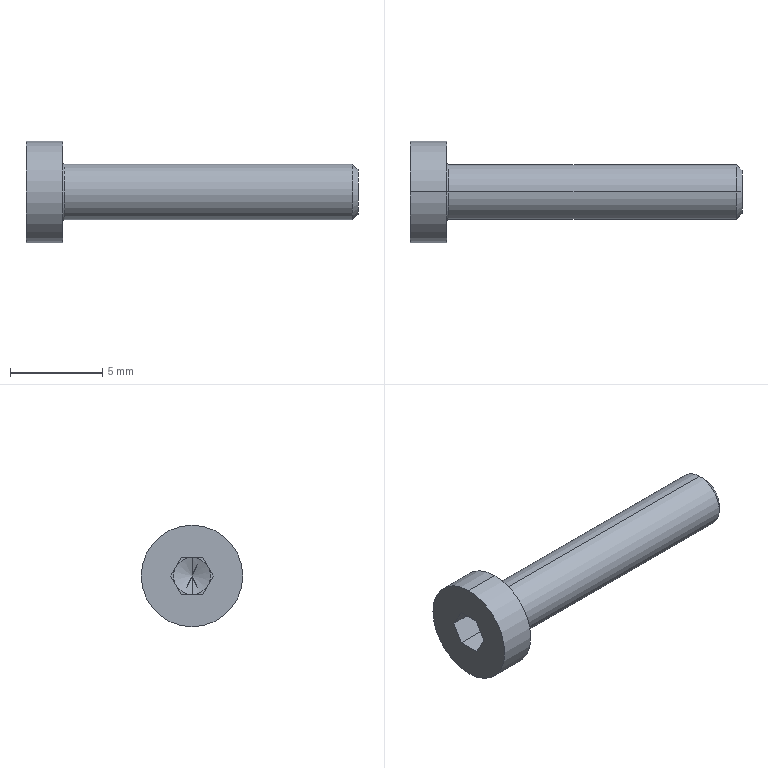Part | SolidWorks | features ICE 1, RevCut 1, Revolution 1 | 1 solid | 25 faces | box 18 x 5.5 x 5.5 mm | volume 154.645 mm3 | plane 15 | cone 4 | cylinder 4 | torus 2 | commonest cylinder face diameters 3 x2 5.5 x2
STEP:
#1=CARTESIAN_POINT('',(-0.136,0.,0.));
#2=VERTEX_POINT('',#1);
#3=CARTESIAN_POINT('',(-0.5,0.,1.));
#4=VERTEX_POINT('',#3);
#5=CARTESIAN_POINT('',(-0.136,0.,0.));
#6=DIRECTION('',(-0.342,0.,0.9397));
#7=VECTOR('',#6,1000.);
#8=LINE('',#5,#7);
#9=EDGE_CURVE('',#2,#4,#8,.T.);
#10=ORIENTED_EDGE('',*,*,#9,.F.);
#11=CARTESIAN_POINT('',(-0.5,0.,-1.));
#12=VERTEX_POINT('',#11);
#13=CARTESIAN_POINT('',(-0.136,0.,0.));
#14=DIRECTION('',(-0.342,0.,-0.9397));
#15=VECTOR('',#14,1000.);
#16=LINE('',#13,#15);
#17=EDGE_CURVE('',#2,#12,#16,.T.);
#18=ORIENTED_EDGE('',*,*,#17,.T.);
#19=CARTESIAN_POINT('',(-0.5,-0.866,-0.5));
#20=VERTEX_POINT('',#19);
#21=CARTESIAN_POINT('',(-0.5,0.,0.));
#22=DIRECTION('',(-1.,0.,0.));
#23=DIRECTION('',(0.,0.,1.));
#24=AXIS2_PLACEMENT_3D('',#21,#22,#23);
#25=CIRCLE('',#24,1.);
#26=EDGE_CURVE('',#12,#20,#25,.T.);
#27=ORIENTED_EDGE('',*,*,#26,.T.);
#28=CARTESIAN_POINT('',(-0.5,-0.866,0.5));
#29=VERTEX_POINT('',#28);
#30=CARTESIAN_POINT('',(-0.5,0.,0.));
#31=DIRECTION('',(-1.,0.,0.));
#32=DIRECTION('',(0.,0.,1.));
#33=AXIS2_PLACEMENT_3D('',#30,#31,#32);
#34=CIRCLE('',#33,1.);
#35=EDGE_CURVE('',#20,#29,#34,.T.);
#36=ORIENTED_EDGE('',*,*,#35,.T.);
#37=CARTESIAN_POINT('',(-0.5,0.,0.));
#38=DIRECTION('',(-1.,0.,0.));
#39=DIRECTION('',(0.,0.,1.));
#40=AXIS2_PLACEMENT_3D('',#37,#38,#39);
#41=CIRCLE('',#40,1.);
#42=EDGE_CURVE('',#29,#4,#41,.T.);
#43=ORIENTED_EDGE('',*,*,#42,.T.);
#44=EDGE_LOOP('',(#10,#18,#27,#36,#43));
#45=FACE_OUTER_BOUND('',#44,.T.);
#46=CARTESIAN_POINT('',(-1000.136,0.,0.));
#47=DIRECTION('',(-1.,0.,0.));
#48=DIRECTION('',(0.,0.,1.));
#49=AXIS2_PLACEMENT_3D('',#46,#47,#48);
#50=CONICAL_SURFACE('',#49,2747.477,1.222);
#51=ADVANCED_FACE('',(#45),#50,.F.);
#52=CARTESIAN_POINT('',(0.,0.,2.75));
#53=VERTEX_POINT('',#52);
#54=CARTESIAN_POINT('',(0.,0.,-2.75));
#55=VERTEX_POINT('',#54);
#56=CARTESIAN_POINT('',(0.,0.,0.));
#57=DIRECTION('',(-1.,0.,0.));
#58=DIRECTION('',(0.,0.,1.));
#59=AXIS2_PLACEMENT_3D('',#56,#57,#58);
#60=CIRCLE('',#59,2.75);
#61=EDGE_CURVE('',#53,#55,#60,.T.);
#62=ORIENTED_EDGE('',*,*,#61,.T.);
#63=CARTESIAN_POINT('',(-2.,0.,-2.75));
#64=VERTEX_POINT('',#63);
#65=CARTESIAN_POINT('',(16.,0.,-2.75));
#66=DIRECTION('',(-1.,0.,0.));
#67=VECTOR('',#66,1000.);
#68=LINE('',#65,#67);
#69=EDGE_CURVE('',#55,#64,#68,.T.);
#70=ORIENTED_EDGE('',*,*,#69,.T.);
#71=CARTESIAN_POINT('',(-2.,0.,2.75));
#72=VERTEX_POINT('',#71);
#73=CARTESIAN_POINT('',(-2.,0.,0.));
#74=DIRECTION('',(-1.,0.,0.));
#75=DIRECTION('',(0.,0.,1.));
#76=AXIS2_PLACEMENT_3D('',#73,#74,#75);
#77=CIRCLE('',#76,2.75);
#78=EDGE_CURVE('',#72,#64,#77,.T.);
#79=ORIENTED_EDGE('',*,*,#78,.F.);
#80=CARTESIAN_POINT('',(16.,0.,2.75));
#81=DIRECTION('',(-1.,0.,0.));
#82=VECTOR('',#81,1000.);
#83=LINE('',#80,#82);
#84=EDGE_CURVE('',#53,#72,#83,.T.);
#85=ORIENTED_EDGE('',*,*,#84,.F.);
#86=EDGE_LOOP('',(#62,#70,#79,#85));
#87=FACE_OUTER_BOUND('',#86,.T.);
#88=CARTESIAN_POINT('',(16.,0.,0.));
#89=DIRECTION('',(-1.,0.,0.));
#90=DIRECTION('',(0.,0.,1.));
#91=AXIS2_PLACEMENT_3D('',#88,#89,#90);
#92=CYLINDRICAL_SURFACE('',#91,2.75);
#93=ADVANCED_FACE('',(#87),#92,.T.);
#94=CARTESIAN_POINT('',(0.,0.,-1.6));
#95=VERTEX_POINT('',#94);
#96=CARTESIAN_POINT('',(0.,0.,1.6));
#97=VERTEX_POINT('',#96);
#98=CARTESIAN_POINT('',(0.,0.,0.));
#99=DIRECTION('',(-1.,0.,0.));
#100=DIRECTION('',(0.,0.,1.));
#101=AXIS2_PLACEMENT_3D('',#98,#99,#100);
#102=CIRCLE('',#101,1.6);
#103=EDGE_CURVE('',#95,#97,#102,.T.);
#104=ORIENTED_EDGE('',*,*,#103,.F.);
#105=CARTESIAN_POINT('',(0.1,0.,-1.5));
#106=VERTEX_POINT('',#105);
#107=CARTESIAN_POINT('',(0.1,0.,-1.6));
#108=DIRECTION('',(0.,1.,0.));
#109=DIRECTION('',(0.,0.,1.));
#110=AXIS2_PLACEMENT_3D('',#107,#108,#109);
#111=CIRCLE('',#110,0.1);
#112=EDGE_CURVE('',#95,#106,#111,.T.);
#113=ORIENTED_EDGE('',*,*,#112,.T.);
#114=CARTESIAN_POINT('',(0.1,0.,1.5));
#115=VERTEX_POINT('',#114);
#116=CARTESIAN_POINT('',(0.1,0.,0.));
#117=DIRECTION('',(-1.,0.,0.));
#118=DIRECTION('',(0.,0.,1.));
#119=AXIS2_PLACEMENT_3D('',#116,#117,#118);
#120=CIRCLE('',#119,1.5);
#121=EDGE_CURVE('',#106,#115,#120,.T.);
#122=ORIENTED_EDGE('',*,*,#121,.T.);
#123=CARTESIAN_POINT('',(0.1,0.,1.6));
#124=DIRECTION('',(0.,-1.,0.));
#125=DIRECTION('',(0.,0.,-1.));
#126=AXIS2_PLACEMENT_3D('',#123,#124,#125);
#127=CIRCLE('',#126,0.1);
#128=EDGE_CURVE('',#97,#115,#127,.T.);
#129=ORIENTED_EDGE('',*,*,#128,.F.);
#130=EDGE_LOOP('',(#104,#113,#122,#129));
#131=FACE_OUTER_BOUND('',#130,.T.);
#132=CARTESIAN_POINT('',(0.1,0.,0.));
#133=DIRECTION('',(-1.,0.,0.));
#134=DIRECTION('',(0.,0.,1.));
#135=AXIS2_PLACEMENT_3D('',#132,#133,#134);
#136=TOROIDAL_SURFACE('',#135,1.6,0.1);
#137=ADVANCED_FACE('',(#131),#136,.F.);
#138=CARTESIAN_POINT('',(15.693,0.,1.5));
#139=VERTEX_POINT('',#138);
#140=CARTESIAN_POINT('',(15.693,0.,-1.5));
#141=VERTEX_POINT('',#140);
#142=CARTESIAN_POINT('',(15.693,0.,0.));
#143=DIRECTION('',(-1.,0.,0.));
#144=DIRECTION('',(0.,0.,1.));
#145=AXIS2_PLACEMENT_3D('',#142,#143,#144);
#146=CIRCLE('',#145,1.5);
#147=EDGE_CURVE('',#139,#141,#146,.T.);
#148=ORIENTED_EDGE('',*,*,#147,.T.);
#149=CARTESIAN_POINT('',(16.,0.,-1.5));
#150=DIRECTION('',(-1.,0.,0.));
#151=VECTOR('',#150,1000.);
#152=LINE('',#149,#151);
#153=EDGE_CURVE('',#141,#106,#152,.T.);
#154=ORIENTED_EDGE('',*,*,#153,.T.);
#155=CARTESIAN_POINT('',(0.1,0.,0.));
#156=DIRECTION('',(-1.,0.,0.));
#157=DIRECTION('',(0.,0.,1.));
#158=AXIS2_PLACEMENT_3D('',#155,#156,#157);
#159=CIRCLE('',#158,1.5);
#160=EDGE_CURVE('',#115,#106,#159,.T.);
#161=ORIENTED_EDGE('',*,*,#160,.F.);
#162=CARTESIAN_POINT('',(16.,0.,1.5));
#163=DIRECTION('',(-1.,0.,0.));
#164=VECTOR('',#163,1000.);
#165=LINE('',#162,#164);
#166=EDGE_CURVE('',#139,#115,#165,.T.);
#167=ORIENTED_EDGE('',*,*,#166,.F.);
#168=EDGE_LOOP('',(#148,#154,#161,#167));
#169=FACE_OUTER_BOUND('',#168,.T.);
#170=CARTESIAN_POINT('',(16.,0.,0.));
#171=DIRECTION('',(-1.,0.,0.));
#172=DIRECTION('',(0.,0.,1.));
#173=AXIS2_PLACEMENT_3D('',#170,#171,#172);
#174=CYLINDRICAL_SURFACE('',#173,1.5);
#175=ADVANCED_FACE('',(#169),#174,.T.);
#176=CARTESIAN_POINT('',(16.,0.,1.194));
#177=VERTEX_POINT('',#176);
#178=CARTESIAN_POINT('',(16.,0.,-1.194));
#179=VERTEX_POINT('',#178);
#180=CARTESIAN_POINT('',(16.,0.,0.));
#181=DIRECTION('',(-1.,0.,0.));
#182=DIRECTION('',(0.,0.,1.));
#183=AXIS2_PLACEMENT_3D('',#180,#181,#182);
#184=CIRCLE('',#183,1.194);
#185=EDGE_CURVE('',#177,#179,#184,.T.);
#186=ORIENTED_EDGE('',*,*,#185,.T.);
#187=CARTESIAN_POINT('',(16.,0.,-1.194));
#188=DIRECTION('',(-0.7071,0.,-0.7071));
#189=VECTOR('',#188,1000.);
#190=LINE('',#187,#189);
#191=EDGE_CURVE('',#179,#141,#190,.T.);
#192=ORIENTED_EDGE('',*,*,#191,.T.);
#193=ORIENTED_EDGE('',*,*,#147,.F.);
#194=CARTESIAN_POINT('',(16.,0.,1.194));
#195=DIRECTION('',(-0.7071,0.,0.7071));
#196=VECTOR('',#195,1000.);
#197=LINE('',#194,#196);
#198=EDGE_CURVE('',#177,#139,#197,.T.);
#199=ORIENTED_EDGE('',*,*,#198,.F.);
#200=EDGE_LOOP('',(#186,#192,#193,#199));
#201=FACE_OUTER_BOUND('',#200,.T.);
#202=CARTESIAN_POINT('',(16.,0.,0.));
#203=DIRECTION('',(-1.,0.,0.));
#204=DIRECTION('',(0.,0.,1.));
#205=AXIS2_PLACEMENT_3D('',#202,#203,#204);
#206=CONICAL_SURFACE('',#205,1.194,0.7854);
#207=ADVANCED_FACE('',(#201),#206,.T.);
#208=ORIENTED_EDGE('',*,*,#78,.T.);
#209=CARTESIAN_POINT('',(-2.,0.,0.));
#210=DIRECTION('',(-1.,0.,0.));
#211=DIRECTION('',(0.,0.,1.));
#212=AXIS2_PLACEMENT_3D('',#209,#210,#211);
#213=CIRCLE('',#212,2.75);
#214=EDGE_CURVE('',#64,#72,#213,.T.);
#215=ORIENTED_EDGE('',*,*,#214,.T.);
#216=EDGE_LOOP('',(#208,#215));
#217=FACE_OUTER_BOUND('',#216,.T.);
#218=CARTESIAN_POINT('',(-2.,-0.5774,1.));
#219=VERTEX_POINT('',#218);
#220=CARTESIAN_POINT('',(-2.,-1.155,0.));
#221=VERTEX_POINT('',#220);
#222=CARTESIAN_POINT('',(-2.,-0.5774,1.));
#223=DIRECTION('',(0.,-0.5,-0.866));
#224=VECTOR('',#223,1000.);
#225=LINE('',#222,#224);
#226=EDGE_CURVE('',#219,#221,#225,.T.);
#227=ORIENTED_EDGE('',*,*,#226,.T.);
#228=CARTESIAN_POINT('',(-2.,-0.5774,-1.));
#229=VERTEX_POINT('',#228);
#230=CARTESIAN_POINT('',(-2.,-1.155,0.));
#231=DIRECTION('',(0.,0.5,-0.866));
#232=VECTOR('',#231,1000.);
#233=LINE('',#230,#232);
#234=EDGE_CURVE('',#221,#229,#233,.T.);
#235=ORIENTED_EDGE('',*,*,#234,.T.);
#236=CARTESIAN_POINT('',(-2.,0.5774,-1.));
#237=VERTEX_POINT('',#236);
#238=CARTESIAN_POINT('',(-2.,-0.5774,-1.));
#239=DIRECTION('',(0.,1.,0.));
#240=VECTOR('',#239,1000.);
#241=LINE('',#238,#240);
#242=EDGE_CURVE('',#229,#237,#241,.T.);
#243=ORIENTED_EDGE('',*,*,#242,.T.);
#244=CARTESIAN_POINT('',(-2.,1.155,0.));
#245=VERTEX_POINT('',#244);
#246=CARTESIAN_POINT('',(-2.,0.5774,-1.));
#247=DIRECTION('',(0.,0.5,0.866));
#248=VECTOR('',#247,1000.);
#249=LINE('',#246,#248);
#250=EDGE_CURVE('',#237,#245,#249,.T.);
#251=ORIENTED_EDGE('',*,*,#250,.T.);
#252=CARTESIAN_POINT('',(-2.,0.5774,1.));
#253=VERTEX_POINT('',#252);
#254=CARTESIAN_POINT('',(-2.,1.155,0.));
#255=DIRECTION('',(0.,-0.5,0.866));
#256=VECTOR('',#255,1000.);
#257=LINE('',#254,#256);
#258=EDGE_CURVE('',#245,#253,#257,.T.);
#259=ORIENTED_EDGE('',*,*,#258,.T.);
#260=CARTESIAN_POINT('',(-2.,0.5774,1.));
#261=DIRECTION('',(0.,-1.,0.));
#262=VECTOR('',#261,1000.);
#263=LINE('',#260,#262);
#264=EDGE_CURVE('',#253,#219,#263,.T.);
#265=ORIENTED_EDGE('',*,*,#264,.T.);
#266=EDGE_LOOP('',(#227,#235,#243,#251,#259,#265));
#267=FACE_BOUND('',#266,.T.);
#268=CARTESIAN_POINT('',(-2.,0.,0.));
#269=DIRECTION('',(1.,0.,0.));
#270=DIRECTION('',(0.,0.,-1.));
#271=AXIS2_PLACEMENT_3D('',#268,#269,#270);
#272=PLANE('',#271);
#273=ADVANCED_FACE('',(#217,#267),#272,.F.);
#274=ORIENTED_EDGE('',*,*,#185,.F.);
#275=CARTESIAN_POINT('',(16.,0.,0.));
#276=DIRECTION('',(-1.,0.,0.));
#277=DIRECTION('',(0.,0.,1.));
#278=AXIS2_PLACEMENT_3D('',#275,#276,#277);
#279=CIRCLE('',#278,1.194);
#280=EDGE_CURVE('',#179,#177,#279,.T.);
#281=ORIENTED_EDGE('',*,*,#280,.F.);
#282=EDGE_LOOP('',(#274,#281));
#283=FACE_OUTER_BOUND('',#282,.T.);
#284=CARTESIAN_POINT('',(16.,1.194,0.));
#285=DIRECTION('',(-1.,0.,0.));
#286=DIRECTION('',(0.,0.,1.));
#287=AXIS2_PLACEMENT_3D('',#284,#285,#286);
#288=PLANE('',#287);
#289=ADVANCED_FACE('',(#283),#288,.F.);
#290=ORIENTED_EDGE('',*,*,#191,.F.);
#291=ORIENTED_EDGE('',*,*,#280,.T.);
#292=ORIENTED_EDGE('',*,*,#198,.T.);
#293=CARTESIAN_POINT('',(15.693,0.,0.));
#294=DIRECTION('',(-1.,0.,0.));
#295=DIRECTION('',(0.,0.,1.));
#296=AXIS2_PLACEMENT_3D('',#293,#294,#295);
#297=CIRCLE('',#296,1.5);
#298=EDGE_CURVE('',#141,#139,#297,.T.);
#299=ORIENTED_EDGE('',*,*,#298,.F.);
#300=EDGE_LOOP('',(#290,#291,#292,#299));
#301=FACE_OUTER_BOUND('',#300,.T.);
#302=CARTESIAN_POINT('',(16.,0.,0.));
#303=DIRECTION('',(-1.,0.,0.));
#304=DIRECTION('',(0.,0.,1.));
#305=AXIS2_PLACEMENT_3D('',#302,#303,#304);
#306=CONICAL_SURFACE('',#305,1.194,0.7854);
#307=ADVANCED_FACE('',(#301),#306,.T.);
#308=ORIENTED_EDGE('',*,*,#153,.F.);
#309=ORIENTED_EDGE('',*,*,#298,.T.);
#310=ORIENTED_EDGE('',*,*,#166,.T.);
#311=ORIENTED_EDGE('',*,*,#121,.F.);
#312=EDGE_LOOP('',(#308,#309,#310,#311));
#313=FACE_OUTER_BOUND('',#312,.T.);
#314=CARTESIAN_POINT('',(16.,0.,0.));
#315=DIRECTION('',(-1.,0.,0.));
#316=DIRECTION('',(0.,0.,1.));
#317=AXIS2_PLACEMENT_3D('',#314,#315,#316);
#318=CYLINDRICAL_SURFACE('',#317,1.5);
#319=ADVANCED_FACE('',(#313),#318,.T.);
#320=ORIENTED_EDGE('',*,*,#112,.F.);
#321=CARTESIAN_POINT('',(0.,0.,0.));
#322=DIRECTION('',(-1.,0.,0.));
#323=DIRECTION('',(0.,0.,1.));
#324=AXIS2_PLACEMENT_3D('',#321,#322,#323);
#325=CIRCLE('',#324,1.6);
#326=EDGE_CURVE('',#97,#95,#325,.T.);
#327=ORIENTED_EDGE('',*,*,#326,.F.);
#328=ORIENTED_EDGE('',*,*,#128,.T.);
#329=ORIENTED_EDGE('',*,*,#160,.T.);
#330=EDGE_LOOP('',(#320,#327,#328,#329));
#331=FACE_OUTER_BOUND('',#330,.T.);
#332=CARTESIAN_POINT('',(0.1,0.,0.));
#333=DIRECTION('',(-1.,0.,0.));
#334=DIRECTION('',(0.,0.,1.));
#335=AXIS2_PLACEMENT_3D('',#332,#333,#334);
#336=TOROIDAL_SURFACE('',#335,1.6,0.1);
#337=ADVANCED_FACE('',(#331),#336,.F.);
#338=ORIENTED_EDGE('',*,*,#61,.F.);
#339=CARTESIAN_POINT('',(0.,0.,0.));
#340=DIRECTION('',(-1.,0.,0.));
#341=DIRECTION('',(0.,0.,1.));
#342=AXIS2_PLACEMENT_3D('',#339,#340,#341);
#343=CIRCLE('',#342,2.75);
#344=EDGE_CURVE('',#55,#53,#343,.T.);
#345=ORIENTED_EDGE('',*,*,#344,.F.);
#346=EDGE_LOOP('',(#338,#345));
#347=FACE_OUTER_BOUND('',#346,.T.);
#348=ORIENTED_EDGE('',*,*,#326,.T.);
#349=ORIENTED_EDGE('',*,*,#103,.T.);
#350=EDGE_LOOP('',(#348,#349));
#351=FACE_BOUND('',#350,.T.);
#352=CARTESIAN_POINT('',(0.,2.75,0.));
#353=DIRECTION('',(-1.,0.,0.));
#354=DIRECTION('',(0.,0.,1.));
#355=AXIS2_PLACEMENT_3D('',#352,#353,#354);
#356=PLANE('',#355);
#357=ADVANCED_FACE('',(#347,#351),#356,.F.);
#358=ORIENTED_EDGE('',*,*,#69,.F.);
#359=ORIENTED_EDGE('',*,*,#344,.T.);
#360=ORIENTED_EDGE('',*,*,#84,.T.);
#361=ORIENTED_EDGE('',*,*,#214,.F.);
#362=EDGE_LOOP('',(#358,#359,#360,#361));
#363=FACE_OUTER_BOUND('',#362,.T.);
#364=CARTESIAN_POINT('',(16.,0.,0.));
#365=DIRECTION('',(-1.,0.,0.));
#366=DIRECTION('',(0.,0.,1.));
#367=AXIS2_PLACEMENT_3D('',#364,#365,#366);
#368=CYLINDRICAL_SURFACE('',#367,2.75);
#369=ADVANCED_FACE('',(#363),#368,.T.);
#370=CARTESIAN_POINT('',(-0.5,1.155,0.));
#371=VERTEX_POINT('',#370);
#372=CARTESIAN_POINT('',(-0.5,0.866,0.5));
#373=VERTEX_POINT('',#372);
#374=CARTESIAN_POINT('',(-0.5,1.155,0.));
#375=DIRECTION('',(0.,-0.5,0.866));
#376=VECTOR('',#375,1000.);
#377=LINE('',#374,#376);
#378=EDGE_CURVE('',#371,#373,#377,.T.);
#379=ORIENTED_EDGE('',*,*,#378,.T.);
#380=CARTESIAN_POINT('',(-0.5,0.5774,1.));
#381=VERTEX_POINT('',#380);
#382=CARTESIAN_POINT('',(-0.5,1.155,0.));
#383=DIRECTION('',(0.,-0.5,0.866));
#384=VECTOR('',#383,1000.);
#385=LINE('',#382,#384);
#386=EDGE_CURVE('',#373,#381,#385,.T.);
#387=ORIENTED_EDGE('',*,*,#386,.T.);
#388=CARTESIAN_POINT('',(-0.5,0.5774,1.));
#389=DIRECTION('',(-1.,0.,0.));
#390=VECTOR('',#389,1000.);
#391=LINE('',#388,#390);
#392=EDGE_CURVE('',#381,#253,#391,.T.);
#393=ORIENTED_EDGE('',*,*,#392,.T.);
#394=ORIENTED_EDGE('',*,*,#258,.F.);
#395=CARTESIAN_POINT('',(-0.5,1.155,0.));
#396=DIRECTION('',(-1.,0.,0.));
#397=VECTOR('',#396,1000.);
#398=LINE('',#395,#397);
#399=EDGE_CURVE('',#371,#245,#398,.T.);
#400=ORIENTED_EDGE('',*,*,#399,.F.);
#401=EDGE_LOOP('',(#379,#387,#393,#394,#400));
#402=FACE_OUTER_BOUND('',#401,.T.);
#403=CARTESIAN_POINT('',(-0.5,1.155,0.));
#404=DIRECTION('',(0.,-0.866,-0.5));
#405=DIRECTION('',(0.,0.5,-0.866));
#406=AXIS2_PLACEMENT_3D('',#403,#404,#405);
#407=PLANE('',#406);
#408=ADVANCED_FACE('',(#402),#407,.T.);
#409=CARTESIAN_POINT('',(-0.5,0.5774,1.));
#410=DIRECTION('',(0.,-1.,0.));
#411=VECTOR('',#410,1000.);
#412=LINE('',#409,#411);
#413=EDGE_CURVE('',#381,#4,#412,.T.);
#414=ORIENTED_EDGE('',*,*,#413,.T.);
#415=CARTESIAN_POINT('',(-0.5,-0.5774,1.));
#416=VERTEX_POINT('',#415);
#417=CARTESIAN_POINT('',(-0.5,0.5774,1.));
#418=DIRECTION('',(0.,-1.,0.));
#419=VECTOR('',#418,1000.);
#420=LINE('',#417,#419);
#421=EDGE_CURVE('',#4,#416,#420,.T.);
#422=ORIENTED_EDGE('',*,*,#421,.T.);
#423=CARTESIAN_POINT('',(-0.5,-0.5774,1.));
#424=DIRECTION('',(-1.,0.,0.));
#425=VECTOR('',#424,1000.);
#426=LINE('',#423,#425);
#427=EDGE_CURVE('',#416,#219,#426,.T.);
#428=ORIENTED_EDGE('',*,*,#427,.T.);
#429=ORIENTED_EDGE('',*,*,#264,.F.);
#430=ORIENTED_EDGE('',*,*,#392,.F.);
#431=EDGE_LOOP('',(#414,#422,#428,#429,#430));
#432=FACE_OUTER_BOUND('',#431,.T.);
#433=CARTESIAN_POINT('',(-0.5,0.5774,1.));
#434=DIRECTION('',(0.,0.,-1.));
#435=DIRECTION('',(-1.,0.,0.));
#436=AXIS2_PLACEMENT_3D('',#433,#434,#435);
#437=PLANE('',#436);
#438=ADVANCED_FACE('',(#432),#437,.T.);
#439=CARTESIAN_POINT('',(-0.5,-0.5774,1.));
#440=DIRECTION('',(0.,-0.5,-0.866));
#441=VECTOR('',#440,1000.);
#442=LINE('',#439,#441);
#443=EDGE_CURVE('',#416,#29,#442,.T.);
#444=ORIENTED_EDGE('',*,*,#443,.T.);
#445=CARTESIAN_POINT('',(-0.5,-1.155,0.));
#446=VERTEX_POINT('',#445);
#447=CARTESIAN_POINT('',(-0.5,-0.5774,1.));
#448=DIRECTION('',(0.,-0.5,-0.866));
#449=VECTOR('',#448,1000.);
#450=LINE('',#447,#449);
#451=EDGE_CURVE('',#29,#446,#450,.T.);
#452=ORIENTED_EDGE('',*,*,#451,.T.);
#453=CARTESIAN_POINT('',(-0.5,-1.155,0.));
#454=DIRECTION('',(-1.,0.,0.));
#455=VECTOR('',#454,1000.);
#456=LINE('',#453,#455);
#457=EDGE_CURVE('',#446,#221,#456,.T.);
#458=ORIENTED_EDGE('',*,*,#457,.T.);
#459=ORIENTED_EDGE('',*,*,#226,.F.);
#460=ORIENTED_EDGE('',*,*,#427,.F.);
#461=EDGE_LOOP('',(#444,#452,#458,#459,#460));
#462=FACE_OUTER_BOUND('',#461,.T.);
#463=CARTESIAN_POINT('',(-0.5,-0.5774,1.));
#464=DIRECTION('',(0.,0.866,-0.5));
#465=DIRECTION('',(0.,0.5,0.866));
#466=AXIS2_PLACEMENT_3D('',#463,#464,#465);
#467=PLANE('',#466);
#468=ADVANCED_FACE('',(#462),#467,.T.);
#469=CARTESIAN_POINT('',(-0.5,-1.155,0.));
#470=DIRECTION('',(0.,0.5,-0.866));
#471=VECTOR('',#470,1000.);
#472=LINE('',#469,#471);
#473=EDGE_CURVE('',#446,#20,#472,.T.);
#474=ORIENTED_EDGE('',*,*,#473,.T.);
#475=CARTESIAN_POINT('',(-0.5,-0.5774,-1.));
#476=VERTEX_POINT('',#475);
#477=CARTESIAN_POINT('',(-0.5,-1.155,0.));
#478=DIRECTION('',(0.,0.5,-0.866));
#479=VECTOR('',#478,1000.);
#480=LINE('',#477,#479);
#481=EDGE_CURVE('',#20,#476,#480,.T.);
#482=ORIENTED_EDGE('',*,*,#481,.T.);
#483=CARTESIAN_POINT('',(-0.5,-0.5774,-1.));
#484=DIRECTION('',(-1.,0.,0.));
#485=VECTOR('',#484,1000.);
#486=LINE('',#483,#485);
#487=EDGE_CURVE('',#476,#229,#486,.T.);
#488=ORIENTED_EDGE('',*,*,#487,.T.);
#489=ORIENTED_EDGE('',*,*,#234,.F.);
#490=ORIENTED_EDGE('',*,*,#457,.F.);
#491=EDGE_LOOP('',(#474,#482,#488,#489,#490));
#492=FACE_OUTER_BOUND('',#491,.T.);
#493=CARTESIAN_POINT('',(-0.5,-1.155,0.));
#494=DIRECTION('',(0.,0.866,0.5));
#495=DIRECTION('',(0.,-0.5,0.866));
#496=AXIS2_PLACEMENT_3D('',#493,#494,#495);
#497=PLANE('',#496);
#498=ADVANCED_FACE('',(#492),#497,.T.);
#499=CARTESIAN_POINT('',(-0.5,-0.5774,-1.));
#500=DIRECTION('',(0.,1.,0.));
#501=VECTOR('',#500,1000.);
#502=LINE('',#499,#501);
#503=EDGE_CURVE('',#476,#12,#502,.T.);
#504=ORIENTED_EDGE('',*,*,#503,.T.);
#505=CARTESIAN_POINT('',(-0.5,0.5774,-1.));
#506=VERTEX_POINT('',#505);
#507=CARTESIAN_POINT('',(-0.5,-0.5774,-1.));
#508=DIRECTION('',(0.,1.,0.));
#509=VECTOR('',#508,1000.);
#510=LINE('',#507,#509);
#511=EDGE_CURVE('',#12,#506,#510,.T.);
#512=ORIENTED_EDGE('',*,*,#511,.T.);
#513=CARTESIAN_POINT('',(-0.5,0.5774,-1.));
#514=DIRECTION('',(-1.,0.,0.));
#515=VECTOR('',#514,1000.);
#516=LINE('',#513,#515);
#517=EDGE_CURVE('',#506,#237,#516,.T.);
#518=ORIENTED_EDGE('',*,*,#517,.T.);
#519=ORIENTED_EDGE('',*,*,#242,.F.);
#520=ORIENTED_EDGE('',*,*,#487,.F.);
#521=EDGE_LOOP('',(#504,#512,#518,#519,#520));
#522=FACE_OUTER_BOUND('',#521,.T.);
#523=CARTESIAN_POINT('',(-0.5,-0.5774,-1.));
#524=DIRECTION('',(0.,0.,1.));
#525=DIRECTION('',(1.,0.,0.));
#526=AXIS2_PLACEMENT_3D('',#523,#524,#525);
#527=PLANE('',#526);
#528=ADVANCED_FACE('',(#522),#527,.T.);
#529=CARTESIAN_POINT('',(-0.5,0.866,-0.5));
#530=VERTEX_POINT('',#529);
#531=CARTESIAN_POINT('',(-0.5,0.5774,-1.));
#532=DIRECTION('',(0.,0.5,0.866));
#533=VECTOR('',#532,1000.);
#534=LINE('',#531,#533);
#535=EDGE_CURVE('',#506,#530,#534,.T.);
#536=ORIENTED_EDGE('',*,*,#535,.T.);
#537=CARTESIAN_POINT('',(-0.5,0.5774,-1.));
#538=DIRECTION('',(0.,0.5,0.866));
#539=VECTOR('',#538,1000.);
#540=LINE('',#537,#539);
#541=EDGE_CURVE('',#530,#371,#540,.T.);
#542=ORIENTED_EDGE('',*,*,#541,.T.);
#543=ORIENTED_EDGE('',*,*,#399,.T.);
#544=ORIENTED_EDGE('',*,*,#250,.F.);
#545=ORIENTED_EDGE('',*,*,#517,.F.);
#546=EDGE_LOOP('',(#536,#542,#543,#544,#545));
#547=FACE_OUTER_BOUND('',#546,.T.);
#548=CARTESIAN_POINT('',(-0.5,0.5774,-1.));
#549=DIRECTION('',(0.,-0.866,0.5));
#550=DIRECTION('',(0.,-0.5,-0.866));
#551=AXIS2_PLACEMENT_3D('',#548,#549,#550);
#552=PLANE('',#551);
#553=ADVANCED_FACE('',(#547),#552,.T.);
#554=CARTESIAN_POINT('',(-0.5,0.,0.));
#555=DIRECTION('',(-1.,0.,0.));
#556=DIRECTION('',(0.,0.,1.));
#557=AXIS2_PLACEMENT_3D('',#554,#555,#556);
#558=CIRCLE('',#557,1.);
#559=EDGE_CURVE('',#530,#12,#558,.T.);
#560=ORIENTED_EDGE('',*,*,#559,.F.);
#561=ORIENTED_EDGE('',*,*,#535,.F.);
#562=ORIENTED_EDGE('',*,*,#511,.F.);
#563=EDGE_LOOP('',(#560,#561,#562));
#564=FACE_OUTER_BOUND('',#563,.T.);
#565=CARTESIAN_POINT('',(-0.5,0.,0.));
#566=DIRECTION('',(1.,0.,0.));
#567=DIRECTION('',(0.,0.,-1.));
#568=AXIS2_PLACEMENT_3D('',#565,#566,#567);
#569=PLANE('',#568);
#570=ADVANCED_FACE('',(#564),#569,.F.);
#571=CARTESIAN_POINT('',(-0.5,0.,0.));
#572=DIRECTION('',(-1.,0.,0.));
#573=DIRECTION('',(0.,0.,1.));
#574=AXIS2_PLACEMENT_3D('',#571,#572,#573);
#575=CIRCLE('',#574,1.);
#576=EDGE_CURVE('',#373,#530,#575,.T.);
#577=ORIENTED_EDGE('',*,*,#576,.F.);
#578=ORIENTED_EDGE('',*,*,#378,.F.);
#579=ORIENTED_EDGE('',*,*,#541,.F.);
#580=EDGE_LOOP('',(#577,#578,#579));
#581=FACE_OUTER_BOUND('',#580,.T.);
#582=CARTESIAN_POINT('',(-0.5,0.,0.));
#583=DIRECTION('',(1.,0.,0.));
#584=DIRECTION('',(0.,0.,-1.));
#585=AXIS2_PLACEMENT_3D('',#582,#583,#584);
#586=PLANE('',#585);
#587=ADVANCED_FACE('',(#581),#586,.F.);
#588=CARTESIAN_POINT('',(-0.5,0.,0.));
#589=DIRECTION('',(-1.,0.,0.));
#590=DIRECTION('',(0.,0.,1.));
#591=AXIS2_PLACEMENT_3D('',#588,#589,#590);
#592=CIRCLE('',#591,1.);
#593=EDGE_CURVE('',#4,#373,#592,.T.);
#594=ORIENTED_EDGE('',*,*,#593,.F.);
#595=ORIENTED_EDGE('',*,*,#413,.F.);
#596=ORIENTED_EDGE('',*,*,#386,.F.);
#597=EDGE_LOOP('',(#594,#595,#596));
#598=FACE_OUTER_BOUND('',#597,.T.);
#599=CARTESIAN_POINT('',(-0.5,0.,0.));
#600=DIRECTION('',(1.,0.,0.));
#601=DIRECTION('',(0.,0.,-1.));
#602=AXIS2_PLACEMENT_3D('',#599,#600,#601);
#603=PLANE('',#602);
#604=ADVANCED_FACE('',(#598),#603,.F.);
#605=ORIENTED_EDGE('',*,*,#42,.F.);
#606=ORIENTED_EDGE('',*,*,#443,.F.);
#607=ORIENTED_EDGE('',*,*,#421,.F.);
#608=EDGE_LOOP('',(#605,#606,#607));
#609=FACE_OUTER_BOUND('',#608,.T.);
#610=CARTESIAN_POINT('',(-0.5,0.,0.));
#611=DIRECTION('',(1.,0.,0.));
#612=DIRECTION('',(0.,0.,-1.));
#613=AXIS2_PLACEMENT_3D('',#610,#611,#612);
#614=PLANE('',#613);
#615=ADVANCED_FACE('',(#609),#614,.F.);
#616=ORIENTED_EDGE('',*,*,#35,.F.);
#617=ORIENTED_EDGE('',*,*,#473,.F.);
#618=ORIENTED_EDGE('',*,*,#451,.F.);
#619=EDGE_LOOP('',(#616,#617,#618));
#620=FACE_OUTER_BOUND('',#619,.T.);
#621=CARTESIAN_POINT('',(-0.5,0.,0.));
#622=DIRECTION('',(1.,0.,0.));
#623=DIRECTION('',(0.,0.,-1.));
#624=AXIS2_PLACEMENT_3D('',#621,#622,#623);
#625=PLANE('',#624);
#626=ADVANCED_FACE('',(#620),#625,.F.);
#627=ORIENTED_EDGE('',*,*,#26,.F.);
#628=ORIENTED_EDGE('',*,*,#503,.F.);
#629=ORIENTED_EDGE('',*,*,#481,.F.);
#630=EDGE_LOOP('',(#627,#628,#629));
#631=FACE_OUTER_BOUND('',#630,.T.);
#632=CARTESIAN_POINT('',(-0.5,0.,0.));
#633=DIRECTION('',(1.,0.,0.));
#634=DIRECTION('',(0.,0.,-1.));
#635=AXIS2_PLACEMENT_3D('',#632,#633,#634);
#636=PLANE('',#635);
#637=ADVANCED_FACE('',(#631),#636,.F.);
#638=ORIENTED_EDGE('',*,*,#17,.F.);
#639=ORIENTED_EDGE('',*,*,#9,.T.);
#640=ORIENTED_EDGE('',*,*,#593,.T.);
#641=ORIENTED_EDGE('',*,*,#576,.T.);
#642=ORIENTED_EDGE('',*,*,#559,.T.);
#643=EDGE_LOOP('',(#638,#639,#640,#641,#642));
#644=FACE_OUTER_BOUND('',#643,.T.);
#645=CARTESIAN_POINT('',(-1000.136,0.,0.));
#646=DIRECTION('',(-1.,0.,0.));
#647=DIRECTION('',(0.,0.,1.));
#648=AXIS2_PLACEMENT_3D('',#645,#646,#647);
#649=CONICAL_SURFACE('',#648,2747.477,1.222);
#650=ADVANCED_FACE('',(#644),#649,.F.);
#651=CLOSED_SHELL('',(#51,#93,#137,#175,#207,#273,#289,#307,#319,#337,#357,#369,#408,#438,#468,#498,#528,#553,#570,#587,#604,#615,#626,#637,#650));
#652=MANIFOLD_SOLID_BREP('',#651);
#653=CARTESIAN_POINT('',(0.,0.,0.));
#654=DIRECTION('',(0.,0.,1.));
#655=DIRECTION('',(1.,0.,0.));
#656=AXIS2_PLACEMENT_3D('',#653,#654,#655);
#657=(LENGTH_UNIT()NAMED_UNIT(*)SI_UNIT(.MILLI.,.METRE.));
#658=UNCERTAINTY_MEASURE_WITH_UNIT(LENGTH_MEASURE(0.00001),#657,'','');
#659=(NAMED_UNIT(*)PLANE_ANGLE_UNIT()SI_UNIT($,.RADIAN.));
#660=(NAMED_UNIT(*)SI_UNIT($,.STERADIAN.)SOLID_ANGLE_UNIT());
#661=(GEOMETRIC_REPRESENTATION_CONTEXT(3)GLOBAL_UNCERTAINTY_ASSIGNED_CONTEXT((#658))GLOBAL_UNIT_ASSIGNED_CONTEXT((#657,#659,#660))REPRESENTATION_CONTEXT('',''));
#662=ADVANCED_BREP_SHAPE_REPRESENTATION('',(#652,#656),#661);